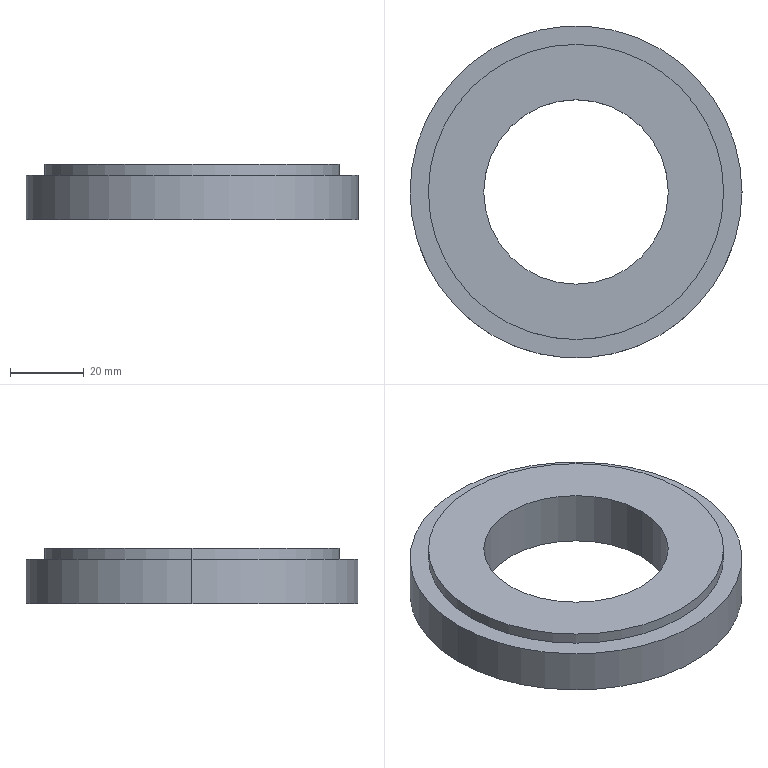Part | SolidWorks | features 3DProfileFeature 1, Extrusion 1, HoleWzd 1, ICE 1 | 1 solid | 33 faces | box 90 x 90 x 15 mm | volume 61433 mm3 | cylinder 18 | cone 12 | plane 3 | commonest cylinder face diameters 3.3 x12 50 x2 80 x2 90 x2
STEP:
#1=CARTESIAN_POINT('',(33.693,18.5,10.1));
#2=VERTEX_POINT('',#1);
#3=CARTESIAN_POINT('',(30.393,18.5,10.1));
#4=VERTEX_POINT('',#3);
#5=CARTESIAN_POINT('',(32.043,18.5,10.1));
#6=DIRECTION('',(0.,0.,-1.));
#7=DIRECTION('',(-1.,0.,0.));
#8=AXIS2_PLACEMENT_3D('',#5,#6,#7);
#9=CIRCLE('',#8,1.65);
#10=EDGE_CURVE('',#2,#4,#9,.T.);
#11=ORIENTED_EDGE('',*,*,#10,.F.);
#12=CARTESIAN_POINT('',(33.693,18.5,0.));
#13=VERTEX_POINT('',#12);
#14=CARTESIAN_POINT('',(33.693,18.5,0.));
#15=DIRECTION('',(0.,0.,-1.));
#16=VECTOR('',#15,1000.);
#17=LINE('',#14,#16);
#18=EDGE_CURVE('',#2,#13,#17,.T.);
#19=ORIENTED_EDGE('',*,*,#18,.T.);
#20=CARTESIAN_POINT('',(30.393,18.5,0.));
#21=VERTEX_POINT('',#20);
#22=CARTESIAN_POINT('',(32.043,18.5,0.));
#23=DIRECTION('',(0.,0.,-1.));
#24=DIRECTION('',(-1.,0.,0.));
#25=AXIS2_PLACEMENT_3D('',#22,#23,#24);
#26=CIRCLE('',#25,1.65);
#27=EDGE_CURVE('',#13,#21,#26,.T.);
#28=ORIENTED_EDGE('',*,*,#27,.T.);
#29=CARTESIAN_POINT('',(30.393,18.5,0.));
#30=DIRECTION('',(0.,0.,-1.));
#31=VECTOR('',#30,1000.);
#32=LINE('',#29,#31);
#33=EDGE_CURVE('',#4,#21,#32,.T.);
#34=ORIENTED_EDGE('',*,*,#33,.F.);
#35=EDGE_LOOP('',(#11,#19,#28,#34));
#36=FACE_OUTER_BOUND('',#35,.T.);
#37=CARTESIAN_POINT('',(32.043,18.5,0.));
#38=DIRECTION('',(0.,0.,-1.));
#39=DIRECTION('',(-1.,0.,0.));
#40=AXIS2_PLACEMENT_3D('',#37,#38,#39);
#41=CYLINDRICAL_SURFACE('',#40,1.65);
#42=ADVANCED_FACE('',(#36),#41,.F.);
#43=CARTESIAN_POINT('',(32.043,18.5,11.091));
#44=VERTEX_POINT('',#43);
#45=CARTESIAN_POINT('',(30.393,18.5,10.1));
#46=DIRECTION('',(-0.8572,0.,-0.515));
#47=VECTOR('',#46,1000.);
#48=LINE('',#45,#47);
#49=EDGE_CURVE('',#44,#4,#48,.T.);
#50=ORIENTED_EDGE('',*,*,#49,.F.);
#51=CARTESIAN_POINT('',(33.693,18.5,10.1));
#52=DIRECTION('',(0.8572,0.,-0.515));
#53=VECTOR('',#52,1000.);
#54=LINE('',#51,#53);
#55=EDGE_CURVE('',#44,#2,#54,.T.);
#56=ORIENTED_EDGE('',*,*,#55,.T.);
#57=ORIENTED_EDGE('',*,*,#10,.T.);
#58=EDGE_LOOP('',(#50,#56,#57));
#59=FACE_OUTER_BOUND('',#58,.T.);
#60=CARTESIAN_POINT('',(32.043,18.5,10.1));
#61=DIRECTION('',(0.,0.,-1.));
#62=DIRECTION('',(-1.,0.,0.));
#63=AXIS2_PLACEMENT_3D('',#60,#61,#62);
#64=CONICAL_SURFACE('',#63,1.65,1.03);
#65=ADVANCED_FACE('',(#59),#64,.F.);
#66=CARTESIAN_POINT('',(1.65,37.,10.1));
#67=VERTEX_POINT('',#66);
#68=CARTESIAN_POINT('',(-1.65,37.,10.1));
#69=VERTEX_POINT('',#68);
#70=CARTESIAN_POINT('',(0.,37.,10.1));
#71=DIRECTION('',(0.,0.,-1.));
#72=DIRECTION('',(-1.,0.,0.));
#73=AXIS2_PLACEMENT_3D('',#70,#71,#72);
#74=CIRCLE('',#73,1.65);
#75=EDGE_CURVE('',#67,#69,#74,.T.);
#76=ORIENTED_EDGE('',*,*,#75,.F.);
#77=CARTESIAN_POINT('',(1.65,37.,0.));
#78=VERTEX_POINT('',#77);
#79=CARTESIAN_POINT('',(1.65,37.,0.));
#80=DIRECTION('',(0.,0.,-1.));
#81=VECTOR('',#80,1000.);
#82=LINE('',#79,#81);
#83=EDGE_CURVE('',#67,#78,#82,.T.);
#84=ORIENTED_EDGE('',*,*,#83,.T.);
#85=CARTESIAN_POINT('',(-1.65,37.,0.));
#86=VERTEX_POINT('',#85);
#87=CARTESIAN_POINT('',(0.,37.,0.));
#88=DIRECTION('',(0.,0.,-1.));
#89=DIRECTION('',(-1.,0.,0.));
#90=AXIS2_PLACEMENT_3D('',#87,#88,#89);
#91=CIRCLE('',#90,1.65);
#92=EDGE_CURVE('',#78,#86,#91,.T.);
#93=ORIENTED_EDGE('',*,*,#92,.T.);
#94=CARTESIAN_POINT('',(-1.65,37.,0.));
#95=DIRECTION('',(0.,0.,-1.));
#96=VECTOR('',#95,1000.);
#97=LINE('',#94,#96);
#98=EDGE_CURVE('',#69,#86,#97,.T.);
#99=ORIENTED_EDGE('',*,*,#98,.F.);
#100=EDGE_LOOP('',(#76,#84,#93,#99));
#101=FACE_OUTER_BOUND('',#100,.T.);
#102=CARTESIAN_POINT('',(0.,37.,0.));
#103=DIRECTION('',(0.,0.,-1.));
#104=DIRECTION('',(-1.,0.,0.));
#105=AXIS2_PLACEMENT_3D('',#102,#103,#104);
#106=CYLINDRICAL_SURFACE('',#105,1.65);
#107=ADVANCED_FACE('',(#101),#106,.F.);
#108=CARTESIAN_POINT('',(0.,37.,11.091));
#109=VERTEX_POINT('',#108);
#110=CARTESIAN_POINT('',(-1.65,37.,10.1));
#111=DIRECTION('',(-0.8572,0.,-0.515));
#112=VECTOR('',#111,1000.);
#113=LINE('',#110,#112);
#114=EDGE_CURVE('',#109,#69,#113,.T.);
#115=ORIENTED_EDGE('',*,*,#114,.F.);
#116=CARTESIAN_POINT('',(1.65,37.,10.1));
#117=DIRECTION('',(0.8572,0.,-0.515));
#118=VECTOR('',#117,1000.);
#119=LINE('',#116,#118);
#120=EDGE_CURVE('',#109,#67,#119,.T.);
#121=ORIENTED_EDGE('',*,*,#120,.T.);
#122=ORIENTED_EDGE('',*,*,#75,.T.);
#123=EDGE_LOOP('',(#115,#121,#122));
#124=FACE_OUTER_BOUND('',#123,.T.);
#125=CARTESIAN_POINT('',(0.,37.,10.1));
#126=DIRECTION('',(0.,0.,-1.));
#127=DIRECTION('',(-1.,0.,0.));
#128=AXIS2_PLACEMENT_3D('',#125,#126,#127);
#129=CONICAL_SURFACE('',#128,1.65,1.03);
#130=ADVANCED_FACE('',(#124),#129,.F.);
#131=CARTESIAN_POINT('',(-30.393,18.5,10.1));
#132=VERTEX_POINT('',#131);
#133=CARTESIAN_POINT('',(-33.693,18.5,10.1));
#134=VERTEX_POINT('',#133);
#135=CARTESIAN_POINT('',(-32.043,18.5,10.1));
#136=DIRECTION('',(0.,0.,-1.));
#137=DIRECTION('',(-1.,0.,0.));
#138=AXIS2_PLACEMENT_3D('',#135,#136,#137);
#139=CIRCLE('',#138,1.65);
#140=EDGE_CURVE('',#132,#134,#139,.T.);
#141=ORIENTED_EDGE('',*,*,#140,.F.);
#142=CARTESIAN_POINT('',(-30.393,18.5,0.));
#143=VERTEX_POINT('',#142);
#144=CARTESIAN_POINT('',(-30.393,18.5,0.));
#145=DIRECTION('',(0.,0.,-1.));
#146=VECTOR('',#145,1000.);
#147=LINE('',#144,#146);
#148=EDGE_CURVE('',#132,#143,#147,.T.);
#149=ORIENTED_EDGE('',*,*,#148,.T.);
#150=CARTESIAN_POINT('',(-33.693,18.5,0.));
#151=VERTEX_POINT('',#150);
#152=CARTESIAN_POINT('',(-32.043,18.5,0.));
#153=DIRECTION('',(0.,0.,-1.));
#154=DIRECTION('',(-1.,0.,0.));
#155=AXIS2_PLACEMENT_3D('',#152,#153,#154);
#156=CIRCLE('',#155,1.65);
#157=EDGE_CURVE('',#143,#151,#156,.T.);
#158=ORIENTED_EDGE('',*,*,#157,.T.);
#159=CARTESIAN_POINT('',(-33.693,18.5,0.));
#160=DIRECTION('',(0.,0.,-1.));
#161=VECTOR('',#160,1000.);
#162=LINE('',#159,#161);
#163=EDGE_CURVE('',#134,#151,#162,.T.);
#164=ORIENTED_EDGE('',*,*,#163,.F.);
#165=EDGE_LOOP('',(#141,#149,#158,#164));
#166=FACE_OUTER_BOUND('',#165,.T.);
#167=CARTESIAN_POINT('',(-32.043,18.5,0.));
#168=DIRECTION('',(0.,0.,-1.));
#169=DIRECTION('',(-1.,0.,0.));
#170=AXIS2_PLACEMENT_3D('',#167,#168,#169);
#171=CYLINDRICAL_SURFACE('',#170,1.65);
#172=ADVANCED_FACE('',(#166),#171,.F.);
#173=CARTESIAN_POINT('',(-32.043,18.5,11.091));
#174=VERTEX_POINT('',#173);
#175=CARTESIAN_POINT('',(-33.693,18.5,10.1));
#176=DIRECTION('',(-0.8572,0.,-0.515));
#177=VECTOR('',#176,1000.);
#178=LINE('',#175,#177);
#179=EDGE_CURVE('',#174,#134,#178,.T.);
#180=ORIENTED_EDGE('',*,*,#179,.F.);
#181=CARTESIAN_POINT('',(-30.393,18.5,10.1));
#182=DIRECTION('',(0.8572,0.,-0.515));
#183=VECTOR('',#182,1000.);
#184=LINE('',#181,#183);
#185=EDGE_CURVE('',#174,#132,#184,.T.);
#186=ORIENTED_EDGE('',*,*,#185,.T.);
#187=ORIENTED_EDGE('',*,*,#140,.T.);
#188=EDGE_LOOP('',(#180,#186,#187));
#189=FACE_OUTER_BOUND('',#188,.T.);
#190=CARTESIAN_POINT('',(-32.043,18.5,10.1));
#191=DIRECTION('',(0.,0.,-1.));
#192=DIRECTION('',(-1.,0.,0.));
#193=AXIS2_PLACEMENT_3D('',#190,#191,#192);
#194=CONICAL_SURFACE('',#193,1.65,1.03);
#195=ADVANCED_FACE('',(#189),#194,.F.);
#196=CARTESIAN_POINT('',(-30.393,-18.5,10.1));
#197=VERTEX_POINT('',#196);
#198=CARTESIAN_POINT('',(-33.693,-18.5,10.1));
#199=VERTEX_POINT('',#198);
#200=CARTESIAN_POINT('',(-32.043,-18.5,10.1));
#201=DIRECTION('',(0.,0.,-1.));
#202=DIRECTION('',(-1.,0.,0.));
#203=AXIS2_PLACEMENT_3D('',#200,#201,#202);
#204=CIRCLE('',#203,1.65);
#205=EDGE_CURVE('',#197,#199,#204,.T.);
#206=ORIENTED_EDGE('',*,*,#205,.F.);
#207=CARTESIAN_POINT('',(-30.393,-18.5,0.));
#208=VERTEX_POINT('',#207);
#209=CARTESIAN_POINT('',(-30.393,-18.5,0.));
#210=DIRECTION('',(0.,0.,-1.));
#211=VECTOR('',#210,1000.);
#212=LINE('',#209,#211);
#213=EDGE_CURVE('',#197,#208,#212,.T.);
#214=ORIENTED_EDGE('',*,*,#213,.T.);
#215=CARTESIAN_POINT('',(-33.693,-18.5,0.));
#216=VERTEX_POINT('',#215);
#217=CARTESIAN_POINT('',(-32.043,-18.5,0.));
#218=DIRECTION('',(0.,0.,-1.));
#219=DIRECTION('',(-1.,0.,0.));
#220=AXIS2_PLACEMENT_3D('',#217,#218,#219);
#221=CIRCLE('',#220,1.65);
#222=EDGE_CURVE('',#208,#216,#221,.T.);
#223=ORIENTED_EDGE('',*,*,#222,.T.);
#224=CARTESIAN_POINT('',(-33.693,-18.5,0.));
#225=DIRECTION('',(0.,0.,-1.));
#226=VECTOR('',#225,1000.);
#227=LINE('',#224,#226);
#228=EDGE_CURVE('',#199,#216,#227,.T.);
#229=ORIENTED_EDGE('',*,*,#228,.F.);
#230=EDGE_LOOP('',(#206,#214,#223,#229));
#231=FACE_OUTER_BOUND('',#230,.T.);
#232=CARTESIAN_POINT('',(-32.043,-18.5,0.));
#233=DIRECTION('',(0.,0.,-1.));
#234=DIRECTION('',(-1.,0.,0.));
#235=AXIS2_PLACEMENT_3D('',#232,#233,#234);
#236=CYLINDRICAL_SURFACE('',#235,1.65);
#237=ADVANCED_FACE('',(#231),#236,.F.);
#238=CARTESIAN_POINT('',(-32.043,-18.5,11.091));
#239=VERTEX_POINT('',#238);
#240=CARTESIAN_POINT('',(-33.693,-18.5,10.1));
#241=DIRECTION('',(-0.8572,0.,-0.515));
#242=VECTOR('',#241,1000.);
#243=LINE('',#240,#242);
#244=EDGE_CURVE('',#239,#199,#243,.T.);
#245=ORIENTED_EDGE('',*,*,#244,.F.);
#246=CARTESIAN_POINT('',(-30.393,-18.5,10.1));
#247=DIRECTION('',(0.8572,0.,-0.515));
#248=VECTOR('',#247,1000.);
#249=LINE('',#246,#248);
#250=EDGE_CURVE('',#239,#197,#249,.T.);
#251=ORIENTED_EDGE('',*,*,#250,.T.);
#252=ORIENTED_EDGE('',*,*,#205,.T.);
#253=EDGE_LOOP('',(#245,#251,#252));
#254=FACE_OUTER_BOUND('',#253,.T.);
#255=CARTESIAN_POINT('',(-32.043,-18.5,10.1));
#256=DIRECTION('',(0.,0.,-1.));
#257=DIRECTION('',(-1.,0.,0.));
#258=AXIS2_PLACEMENT_3D('',#255,#256,#257);
#259=CONICAL_SURFACE('',#258,1.65,1.03);
#260=ADVANCED_FACE('',(#254),#259,.F.);
#261=CARTESIAN_POINT('',(1.65,-37.,10.1));
#262=VERTEX_POINT('',#261);
#263=CARTESIAN_POINT('',(-1.65,-37.,10.1));
#264=VERTEX_POINT('',#263);
#265=CARTESIAN_POINT('',(0.,-37.,10.1));
#266=DIRECTION('',(0.,0.,-1.));
#267=DIRECTION('',(-1.,0.,0.));
#268=AXIS2_PLACEMENT_3D('',#265,#266,#267);
#269=CIRCLE('',#268,1.65);
#270=EDGE_CURVE('',#262,#264,#269,.T.);
#271=ORIENTED_EDGE('',*,*,#270,.F.);
#272=CARTESIAN_POINT('',(1.65,-37.,0.));
#273=VERTEX_POINT('',#272);
#274=CARTESIAN_POINT('',(1.65,-37.,0.));
#275=DIRECTION('',(0.,0.,-1.));
#276=VECTOR('',#275,1000.);
#277=LINE('',#274,#276);
#278=EDGE_CURVE('',#262,#273,#277,.T.);
#279=ORIENTED_EDGE('',*,*,#278,.T.);
#280=CARTESIAN_POINT('',(-1.65,-37.,0.));
#281=VERTEX_POINT('',#280);
#282=CARTESIAN_POINT('',(0.,-37.,0.));
#283=DIRECTION('',(0.,0.,-1.));
#284=DIRECTION('',(-1.,0.,0.));
#285=AXIS2_PLACEMENT_3D('',#282,#283,#284);
#286=CIRCLE('',#285,1.65);
#287=EDGE_CURVE('',#273,#281,#286,.T.);
#288=ORIENTED_EDGE('',*,*,#287,.T.);
#289=CARTESIAN_POINT('',(-1.65,-37.,0.));
#290=DIRECTION('',(0.,0.,-1.));
#291=VECTOR('',#290,1000.);
#292=LINE('',#289,#291);
#293=EDGE_CURVE('',#264,#281,#292,.T.);
#294=ORIENTED_EDGE('',*,*,#293,.F.);
#295=EDGE_LOOP('',(#271,#279,#288,#294));
#296=FACE_OUTER_BOUND('',#295,.T.);
#297=CARTESIAN_POINT('',(0.,-37.,0.));
#298=DIRECTION('',(0.,0.,-1.));
#299=DIRECTION('',(-1.,0.,0.));
#300=AXIS2_PLACEMENT_3D('',#297,#298,#299);
#301=CYLINDRICAL_SURFACE('',#300,1.65);
#302=ADVANCED_FACE('',(#296),#301,.F.);
#303=CARTESIAN_POINT('',(0.,-37.,11.091));
#304=VERTEX_POINT('',#303);
#305=CARTESIAN_POINT('',(-1.65,-37.,10.1));
#306=DIRECTION('',(-0.8572,0.,-0.515));
#307=VECTOR('',#306,1000.);
#308=LINE('',#305,#307);
#309=EDGE_CURVE('',#304,#264,#308,.T.);
#310=ORIENTED_EDGE('',*,*,#309,.F.);
#311=CARTESIAN_POINT('',(1.65,-37.,10.1));
#312=DIRECTION('',(0.8572,0.,-0.515));
#313=VECTOR('',#312,1000.);
#314=LINE('',#311,#313);
#315=EDGE_CURVE('',#304,#262,#314,.T.);
#316=ORIENTED_EDGE('',*,*,#315,.T.);
#317=ORIENTED_EDGE('',*,*,#270,.T.);
#318=EDGE_LOOP('',(#310,#316,#317));
#319=FACE_OUTER_BOUND('',#318,.T.);
#320=CARTESIAN_POINT('',(0.,-37.,10.1));
#321=DIRECTION('',(0.,0.,-1.));
#322=DIRECTION('',(-1.,0.,0.));
#323=AXIS2_PLACEMENT_3D('',#320,#321,#322);
#324=CONICAL_SURFACE('',#323,1.65,1.03);
#325=ADVANCED_FACE('',(#319),#324,.F.);
#326=CARTESIAN_POINT('',(33.693,-18.5,10.1));
#327=VERTEX_POINT('',#326);
#328=CARTESIAN_POINT('',(30.393,-18.5,10.1));
#329=VERTEX_POINT('',#328);
#330=CARTESIAN_POINT('',(32.043,-18.5,10.1));
#331=DIRECTION('',(0.,0.,-1.));
#332=DIRECTION('',(-1.,0.,0.));
#333=AXIS2_PLACEMENT_3D('',#330,#331,#332);
#334=CIRCLE('',#333,1.65);
#335=EDGE_CURVE('',#327,#329,#334,.T.);
#336=ORIENTED_EDGE('',*,*,#335,.F.);
#337=CARTESIAN_POINT('',(33.693,-18.5,0.));
#338=VERTEX_POINT('',#337);
#339=CARTESIAN_POINT('',(33.693,-18.5,0.));
#340=DIRECTION('',(0.,0.,-1.));
#341=VECTOR('',#340,1000.);
#342=LINE('',#339,#341);
#343=EDGE_CURVE('',#327,#338,#342,.T.);
#344=ORIENTED_EDGE('',*,*,#343,.T.);
#345=CARTESIAN_POINT('',(30.393,-18.5,0.));
#346=VERTEX_POINT('',#345);
#347=CARTESIAN_POINT('',(32.043,-18.5,0.));
#348=DIRECTION('',(0.,0.,-1.));
#349=DIRECTION('',(-1.,0.,0.));
#350=AXIS2_PLACEMENT_3D('',#347,#348,#349);
#351=CIRCLE('',#350,1.65);
#352=EDGE_CURVE('',#338,#346,#351,.T.);
#353=ORIENTED_EDGE('',*,*,#352,.T.);
#354=CARTESIAN_POINT('',(30.393,-18.5,0.));
#355=DIRECTION('',(0.,0.,-1.));
#356=VECTOR('',#355,1000.);
#357=LINE('',#354,#356);
#358=EDGE_CURVE('',#329,#346,#357,.T.);
#359=ORIENTED_EDGE('',*,*,#358,.F.);
#360=EDGE_LOOP('',(#336,#344,#353,#359));
#361=FACE_OUTER_BOUND('',#360,.T.);
#362=CARTESIAN_POINT('',(32.043,-18.5,0.));
#363=DIRECTION('',(0.,0.,-1.));
#364=DIRECTION('',(-1.,0.,0.));
#365=AXIS2_PLACEMENT_3D('',#362,#363,#364);
#366=CYLINDRICAL_SURFACE('',#365,1.65);
#367=ADVANCED_FACE('',(#361),#366,.F.);
#368=CARTESIAN_POINT('',(32.043,-18.5,11.091));
#369=VERTEX_POINT('',#368);
#370=CARTESIAN_POINT('',(30.393,-18.5,10.1));
#371=DIRECTION('',(-0.8572,0.,-0.515));
#372=VECTOR('',#371,1000.);
#373=LINE('',#370,#372);
#374=EDGE_CURVE('',#369,#329,#373,.T.);
#375=ORIENTED_EDGE('',*,*,#374,.F.);
#376=CARTESIAN_POINT('',(33.693,-18.5,10.1));
#377=DIRECTION('',(0.8572,0.,-0.515));
#378=VECTOR('',#377,1000.);
#379=LINE('',#376,#378);
#380=EDGE_CURVE('',#369,#327,#379,.T.);
#381=ORIENTED_EDGE('',*,*,#380,.T.);
#382=ORIENTED_EDGE('',*,*,#335,.T.);
#383=EDGE_LOOP('',(#375,#381,#382));
#384=FACE_OUTER_BOUND('',#383,.T.);
#385=CARTESIAN_POINT('',(32.043,-18.5,10.1));
#386=DIRECTION('',(0.,0.,-1.));
#387=DIRECTION('',(-1.,0.,0.));
#388=AXIS2_PLACEMENT_3D('',#385,#386,#387);
#389=CONICAL_SURFACE('',#388,1.65,1.03);
#390=ADVANCED_FACE('',(#384),#389,.F.);
#391=CARTESIAN_POINT('',(40.,0.,15.));
#392=VERTEX_POINT('',#391);
#393=CARTESIAN_POINT('',(-40.,0.,15.));
#394=VERTEX_POINT('',#393);
#395=CARTESIAN_POINT('',(0.,0.,15.));
#396=DIRECTION('',(0.,0.,1.));
#397=DIRECTION('',(1.,0.,0.));
#398=AXIS2_PLACEMENT_3D('',#395,#396,#397);
#399=CIRCLE('',#398,40.);
#400=EDGE_CURVE('',#392,#394,#399,.T.);
#401=ORIENTED_EDGE('',*,*,#400,.F.);
#402=CARTESIAN_POINT('',(40.,0.,12.));
#403=VERTEX_POINT('',#402);
#404=CARTESIAN_POINT('',(40.,0.,15.));
#405=DIRECTION('',(0.,0.,-1.));
#406=VECTOR('',#405,1000.);
#407=LINE('',#404,#406);
#408=EDGE_CURVE('',#392,#403,#407,.T.);
#409=ORIENTED_EDGE('',*,*,#408,.T.);
#410=CARTESIAN_POINT('',(-40.,0.,12.));
#411=VERTEX_POINT('',#410);
#412=CARTESIAN_POINT('',(0.,0.,12.));
#413=DIRECTION('',(0.,0.,1.));
#414=DIRECTION('',(1.,0.,0.));
#415=AXIS2_PLACEMENT_3D('',#412,#413,#414);
#416=CIRCLE('',#415,40.);
#417=EDGE_CURVE('',#403,#411,#416,.T.);
#418=ORIENTED_EDGE('',*,*,#417,.T.);
#419=CARTESIAN_POINT('',(-40.,0.,15.));
#420=DIRECTION('',(0.,0.,-1.));
#421=VECTOR('',#420,1000.);
#422=LINE('',#419,#421);
#423=EDGE_CURVE('',#394,#411,#422,.T.);
#424=ORIENTED_EDGE('',*,*,#423,.F.);
#425=EDGE_LOOP('',(#401,#409,#418,#424));
#426=FACE_OUTER_BOUND('',#425,.T.);
#427=CARTESIAN_POINT('',(0.,0.,15.));
#428=DIRECTION('',(0.,0.,-1.));
#429=DIRECTION('',(-1.,0.,0.));
#430=AXIS2_PLACEMENT_3D('',#427,#428,#429);
#431=CYLINDRICAL_SURFACE('',#430,40.);
#432=ADVANCED_FACE('',(#426),#431,.T.);
#433=CARTESIAN_POINT('',(-25.,0.,15.));
#434=VERTEX_POINT('',#433);
#435=CARTESIAN_POINT('',(25.,0.,15.));
#436=VERTEX_POINT('',#435);
#437=CARTESIAN_POINT('',(0.,0.,15.));
#438=DIRECTION('',(0.,0.,1.));
#439=DIRECTION('',(1.,0.,0.));
#440=AXIS2_PLACEMENT_3D('',#437,#438,#439);
#441=CIRCLE('',#440,25.);
#442=EDGE_CURVE('',#434,#436,#441,.T.);
#443=ORIENTED_EDGE('',*,*,#442,.T.);
#444=CARTESIAN_POINT('',(25.,0.,0.));
#445=VERTEX_POINT('',#444);
#446=CARTESIAN_POINT('',(25.,0.,12.));
#447=DIRECTION('',(0.,0.,-1.));
#448=VECTOR('',#447,1000.);
#449=LINE('',#446,#448);
#450=EDGE_CURVE('',#436,#445,#449,.T.);
#451=ORIENTED_EDGE('',*,*,#450,.T.);
#452=CARTESIAN_POINT('',(-25.,0.,0.));
#453=VERTEX_POINT('',#452);
#454=CARTESIAN_POINT('',(0.,0.,0.));
#455=DIRECTION('',(0.,0.,1.));
#456=DIRECTION('',(1.,0.,0.));
#457=AXIS2_PLACEMENT_3D('',#454,#455,#456);
#458=CIRCLE('',#457,25.);
#459=EDGE_CURVE('',#453,#445,#458,.T.);
#460=ORIENTED_EDGE('',*,*,#459,.F.);
#461=CARTESIAN_POINT('',(-25.,0.,12.));
#462=DIRECTION('',(0.,0.,-1.));
#463=VECTOR('',#462,1000.);
#464=LINE('',#461,#463);
#465=EDGE_CURVE('',#434,#453,#464,.T.);
#466=ORIENTED_EDGE('',*,*,#465,.F.);
#467=EDGE_LOOP('',(#443,#451,#460,#466));
#468=FACE_OUTER_BOUND('',#467,.T.);
#469=CARTESIAN_POINT('',(0.,0.,12.));
#470=DIRECTION('',(0.,0.,-1.));
#471=DIRECTION('',(-1.,0.,0.));
#472=AXIS2_PLACEMENT_3D('',#469,#470,#471);
#473=CYLINDRICAL_SURFACE('',#472,25.);
#474=ADVANCED_FACE('',(#468),#473,.F.);
#475=CARTESIAN_POINT('',(45.,0.,12.));
#476=VERTEX_POINT('',#475);
#477=CARTESIAN_POINT('',(-45.,0.,12.));
#478=VERTEX_POINT('',#477);
#479=CARTESIAN_POINT('',(0.,0.,12.));
#480=DIRECTION('',(0.,0.,1.));
#481=DIRECTION('',(1.,0.,0.));
#482=AXIS2_PLACEMENT_3D('',#479,#480,#481);
#483=CIRCLE('',#482,45.);
#484=EDGE_CURVE('',#476,#478,#483,.T.);
#485=ORIENTED_EDGE('',*,*,#484,.F.);
#486=CARTESIAN_POINT('',(45.,0.,0.));
#487=VERTEX_POINT('',#486);
#488=CARTESIAN_POINT('',(45.,0.,12.));
#489=DIRECTION('',(0.,0.,-1.));
#490=VECTOR('',#489,1000.);
#491=LINE('',#488,#490);
#492=EDGE_CURVE('',#476,#487,#491,.T.);
#493=ORIENTED_EDGE('',*,*,#492,.T.);
#494=CARTESIAN_POINT('',(-45.,0.,0.));
#495=VERTEX_POINT('',#494);
#496=CARTESIAN_POINT('',(0.,0.,0.));
#497=DIRECTION('',(0.,0.,1.));
#498=DIRECTION('',(1.,0.,0.));
#499=AXIS2_PLACEMENT_3D('',#496,#497,#498);
#500=CIRCLE('',#499,45.);
#501=EDGE_CURVE('',#487,#495,#500,.T.);
#502=ORIENTED_EDGE('',*,*,#501,.T.);
#503=CARTESIAN_POINT('',(-45.,0.,12.));
#504=DIRECTION('',(0.,0.,-1.));
#505=VECTOR('',#504,1000.);
#506=LINE('',#503,#505);
#507=EDGE_CURVE('',#478,#495,#506,.T.);
#508=ORIENTED_EDGE('',*,*,#507,.F.);
#509=EDGE_LOOP('',(#485,#493,#502,#508));
#510=FACE_OUTER_BOUND('',#509,.T.);
#511=CARTESIAN_POINT('',(0.,0.,12.));
#512=DIRECTION('',(0.,0.,-1.));
#513=DIRECTION('',(-1.,0.,0.));
#514=AXIS2_PLACEMENT_3D('',#511,#512,#513);
#515=CYLINDRICAL_SURFACE('',#514,45.);
#516=ADVANCED_FACE('',(#510),#515,.T.);
#517=CARTESIAN_POINT('',(0.,0.,12.));
#518=DIRECTION('',(0.,0.,1.));
#519=DIRECTION('',(1.,0.,0.));
#520=AXIS2_PLACEMENT_3D('',#517,#518,#519);
#521=CIRCLE('',#520,45.);
#522=EDGE_CURVE('',#478,#476,#521,.T.);
#523=ORIENTED_EDGE('',*,*,#522,.T.);
#524=ORIENTED_EDGE('',*,*,#484,.T.);
#525=EDGE_LOOP('',(#523,#524));
#526=FACE_OUTER_BOUND('',#525,.T.);
#527=CARTESIAN_POINT('',(0.,0.,12.));
#528=DIRECTION('',(0.,0.,1.));
#529=DIRECTION('',(1.,0.,0.));
#530=AXIS2_PLACEMENT_3D('',#527,#528,#529);
#531=CIRCLE('',#530,40.);
#532=EDGE_CURVE('',#411,#403,#531,.T.);
#533=ORIENTED_EDGE('',*,*,#532,.F.);
#534=ORIENTED_EDGE('',*,*,#417,.F.);
#535=EDGE_LOOP('',(#533,#534));
#536=FACE_BOUND('',#535,.T.);
#537=CARTESIAN_POINT('',(0.,0.,12.));
#538=DIRECTION('',(0.,0.,1.));
#539=DIRECTION('',(1.,0.,0.));
#540=AXIS2_PLACEMENT_3D('',#537,#538,#539);
#541=PLANE('',#540);
#542=ADVANCED_FACE('',(#526,#536),#541,.T.);
#543=CARTESIAN_POINT('',(32.043,18.5,0.));
#544=DIRECTION('',(0.,0.,-1.));
#545=DIRECTION('',(-1.,0.,0.));
#546=AXIS2_PLACEMENT_3D('',#543,#544,#545);
#547=CIRCLE('',#546,1.65);
#548=EDGE_CURVE('',#21,#13,#547,.T.);
#549=ORIENTED_EDGE('',*,*,#548,.F.);
#550=ORIENTED_EDGE('',*,*,#27,.F.);
#551=EDGE_LOOP('',(#549,#550));
#552=FACE_BOUND('',#551,.T.);
#553=CARTESIAN_POINT('',(0.,37.,0.));
#554=DIRECTION('',(0.,0.,-1.));
#555=DIRECTION('',(-1.,0.,0.));
#556=AXIS2_PLACEMENT_3D('',#553,#554,#555);
#557=CIRCLE('',#556,1.65);
#558=EDGE_CURVE('',#86,#78,#557,.T.);
#559=ORIENTED_EDGE('',*,*,#558,.F.);
#560=ORIENTED_EDGE('',*,*,#92,.F.);
#561=EDGE_LOOP('',(#559,#560));
#562=FACE_BOUND('',#561,.T.);
#563=CARTESIAN_POINT('',(-32.043,18.5,0.));
#564=DIRECTION('',(0.,0.,-1.));
#565=DIRECTION('',(-1.,0.,0.));
#566=AXIS2_PLACEMENT_3D('',#563,#564,#565);
#567=CIRCLE('',#566,1.65);
#568=EDGE_CURVE('',#151,#143,#567,.T.);
#569=ORIENTED_EDGE('',*,*,#568,.F.);
#570=ORIENTED_EDGE('',*,*,#157,.F.);
#571=EDGE_LOOP('',(#569,#570));
#572=FACE_BOUND('',#571,.T.);
#573=CARTESIAN_POINT('',(-32.043,-18.5,0.));
#574=DIRECTION('',(0.,0.,-1.));
#575=DIRECTION('',(-1.,0.,0.));
#576=AXIS2_PLACEMENT_3D('',#573,#574,#575);
#577=CIRCLE('',#576,1.65);
#578=EDGE_CURVE('',#216,#208,#577,.T.);
#579=ORIENTED_EDGE('',*,*,#578,.F.);
#580=ORIENTED_EDGE('',*,*,#222,.F.);
#581=EDGE_LOOP('',(#579,#580));
#582=FACE_BOUND('',#581,.T.);
#583=CARTESIAN_POINT('',(0.,-37.,0.));
#584=DIRECTION('',(0.,0.,-1.));
#585=DIRECTION('',(-1.,0.,0.));
#586=AXIS2_PLACEMENT_3D('',#583,#584,#585);
#587=CIRCLE('',#586,1.65);
#588=EDGE_CURVE('',#281,#273,#587,.T.);
#589=ORIENTED_EDGE('',*,*,#588,.F.);
#590=ORIENTED_EDGE('',*,*,#287,.F.);
#591=EDGE_LOOP('',(#589,#590));
#592=FACE_BOUND('',#591,.T.);
#593=CARTESIAN_POINT('',(32.043,-18.5,0.));
#594=DIRECTION('',(0.,0.,-1.));
#595=DIRECTION('',(-1.,0.,0.));
#596=AXIS2_PLACEMENT_3D('',#593,#594,#595);
#597=CIRCLE('',#596,1.65);
#598=EDGE_CURVE('',#346,#338,#597,.T.);
#599=ORIENTED_EDGE('',*,*,#598,.F.);
#600=ORIENTED_EDGE('',*,*,#352,.F.);
#601=EDGE_LOOP('',(#599,#600));
#602=FACE_BOUND('',#601,.T.);
#603=CARTESIAN_POINT('',(0.,0.,0.));
#604=DIRECTION('',(0.,0.,1.));
#605=DIRECTION('',(1.,0.,0.));
#606=AXIS2_PLACEMENT_3D('',#603,#604,#605);
#607=CIRCLE('',#606,45.);
#608=EDGE_CURVE('',#495,#487,#607,.T.);
#609=ORIENTED_EDGE('',*,*,#608,.F.);
#610=ORIENTED_EDGE('',*,*,#501,.F.);
#611=EDGE_LOOP('',(#609,#610));
#612=FACE_OUTER_BOUND('',#611,.T.);
#613=ORIENTED_EDGE('',*,*,#459,.T.);
#614=CARTESIAN_POINT('',(0.,0.,0.));
#615=DIRECTION('',(0.,0.,1.));
#616=DIRECTION('',(1.,0.,0.));
#617=AXIS2_PLACEMENT_3D('',#614,#615,#616);
#618=CIRCLE('',#617,25.);
#619=EDGE_CURVE('',#445,#453,#618,.T.);
#620=ORIENTED_EDGE('',*,*,#619,.T.);
#621=EDGE_LOOP('',(#613,#620));
#622=FACE_BOUND('',#621,.T.);
#623=CARTESIAN_POINT('',(0.,0.,0.));
#624=DIRECTION('',(0.,0.,1.));
#625=DIRECTION('',(1.,0.,0.));
#626=AXIS2_PLACEMENT_3D('',#623,#624,#625);
#627=PLANE('',#626);
#628=ADVANCED_FACE('',(#552,#562,#572,#582,#592,#602,#612,#622),#627,.F.);
#629=ORIENTED_EDGE('',*,*,#492,.F.);
#630=ORIENTED_EDGE('',*,*,#522,.F.);
#631=ORIENTED_EDGE('',*,*,#507,.T.);
#632=ORIENTED_EDGE('',*,*,#608,.T.);
#633=EDGE_LOOP('',(#629,#630,#631,#632));
#634=FACE_OUTER_BOUND('',#633,.T.);
#635=CARTESIAN_POINT('',(0.,0.,12.));
#636=DIRECTION('',(0.,0.,-1.));
#637=DIRECTION('',(-1.,0.,0.));
#638=AXIS2_PLACEMENT_3D('',#635,#636,#637);
#639=CYLINDRICAL_SURFACE('',#638,45.);
#640=ADVANCED_FACE('',(#634),#639,.T.);
#641=ORIENTED_EDGE('',*,*,#450,.F.);
#642=CARTESIAN_POINT('',(0.,0.,15.));
#643=DIRECTION('',(0.,0.,1.));
#644=DIRECTION('',(1.,0.,0.));
#645=AXIS2_PLACEMENT_3D('',#642,#643,#644);
#646=CIRCLE('',#645,25.);
#647=EDGE_CURVE('',#436,#434,#646,.T.);
#648=ORIENTED_EDGE('',*,*,#647,.T.);
#649=ORIENTED_EDGE('',*,*,#465,.T.);
#650=ORIENTED_EDGE('',*,*,#619,.F.);
#651=EDGE_LOOP('',(#641,#648,#649,#650));
#652=FACE_OUTER_BOUND('',#651,.T.);
#653=CARTESIAN_POINT('',(0.,0.,12.));
#654=DIRECTION('',(0.,0.,-1.));
#655=DIRECTION('',(-1.,0.,0.));
#656=AXIS2_PLACEMENT_3D('',#653,#654,#655);
#657=CYLINDRICAL_SURFACE('',#656,25.);
#658=ADVANCED_FACE('',(#652),#657,.F.);
#659=CARTESIAN_POINT('',(0.,0.,15.));
#660=DIRECTION('',(0.,0.,1.));
#661=DIRECTION('',(1.,0.,0.));
#662=AXIS2_PLACEMENT_3D('',#659,#660,#661);
#663=CIRCLE('',#662,40.);
#664=EDGE_CURVE('',#394,#392,#663,.T.);
#665=ORIENTED_EDGE('',*,*,#664,.T.);
#666=ORIENTED_EDGE('',*,*,#400,.T.);
#667=EDGE_LOOP('',(#665,#666));
#668=FACE_OUTER_BOUND('',#667,.T.);
#669=ORIENTED_EDGE('',*,*,#442,.F.);
#670=ORIENTED_EDGE('',*,*,#647,.F.);
#671=EDGE_LOOP('',(#669,#670));
#672=FACE_BOUND('',#671,.T.);
#673=CARTESIAN_POINT('',(0.,0.,15.));
#674=DIRECTION('',(0.,0.,1.));
#675=DIRECTION('',(1.,0.,0.));
#676=AXIS2_PLACEMENT_3D('',#673,#674,#675);
#677=PLANE('',#676);
#678=ADVANCED_FACE('',(#668,#672),#677,.T.);
#679=ORIENTED_EDGE('',*,*,#408,.F.);
#680=ORIENTED_EDGE('',*,*,#664,.F.);
#681=ORIENTED_EDGE('',*,*,#423,.T.);
#682=ORIENTED_EDGE('',*,*,#532,.T.);
#683=EDGE_LOOP('',(#679,#680,#681,#682));
#684=FACE_OUTER_BOUND('',#683,.T.);
#685=CARTESIAN_POINT('',(0.,0.,15.));
#686=DIRECTION('',(0.,0.,-1.));
#687=DIRECTION('',(-1.,0.,0.));
#688=AXIS2_PLACEMENT_3D('',#685,#686,#687);
#689=CYLINDRICAL_SURFACE('',#688,40.);
#690=ADVANCED_FACE('',(#684),#689,.T.);
#691=ORIENTED_EDGE('',*,*,#380,.F.);
#692=ORIENTED_EDGE('',*,*,#374,.T.);
#693=CARTESIAN_POINT('',(32.043,-18.5,10.1));
#694=DIRECTION('',(0.,0.,-1.));
#695=DIRECTION('',(-1.,0.,0.));
#696=AXIS2_PLACEMENT_3D('',#693,#694,#695);
#697=CIRCLE('',#696,1.65);
#698=EDGE_CURVE('',#329,#327,#697,.T.);
#699=ORIENTED_EDGE('',*,*,#698,.T.);
#700=EDGE_LOOP('',(#691,#692,#699));
#701=FACE_OUTER_BOUND('',#700,.T.);
#702=CARTESIAN_POINT('',(32.043,-18.5,10.1));
#703=DIRECTION('',(0.,0.,-1.));
#704=DIRECTION('',(-1.,0.,0.));
#705=AXIS2_PLACEMENT_3D('',#702,#703,#704);
#706=CONICAL_SURFACE('',#705,1.65,1.03);
#707=ADVANCED_FACE('',(#701),#706,.F.);
#708=ORIENTED_EDGE('',*,*,#343,.F.);
#709=ORIENTED_EDGE('',*,*,#698,.F.);
#710=ORIENTED_EDGE('',*,*,#358,.T.);
#711=ORIENTED_EDGE('',*,*,#598,.T.);
#712=EDGE_LOOP('',(#708,#709,#710,#711));
#713=FACE_OUTER_BOUND('',#712,.T.);
#714=CARTESIAN_POINT('',(32.043,-18.5,0.));
#715=DIRECTION('',(0.,0.,-1.));
#716=DIRECTION('',(-1.,0.,0.));
#717=AXIS2_PLACEMENT_3D('',#714,#715,#716);
#718=CYLINDRICAL_SURFACE('',#717,1.65);
#719=ADVANCED_FACE('',(#713),#718,.F.);
#720=ORIENTED_EDGE('',*,*,#315,.F.);
#721=ORIENTED_EDGE('',*,*,#309,.T.);
#722=CARTESIAN_POINT('',(0.,-37.,10.1));
#723=DIRECTION('',(0.,0.,-1.));
#724=DIRECTION('',(-1.,0.,0.));
#725=AXIS2_PLACEMENT_3D('',#722,#723,#724);
#726=CIRCLE('',#725,1.65);
#727=EDGE_CURVE('',#264,#262,#726,.T.);
#728=ORIENTED_EDGE('',*,*,#727,.T.);
#729=EDGE_LOOP('',(#720,#721,#728));
#730=FACE_OUTER_BOUND('',#729,.T.);
#731=CARTESIAN_POINT('',(0.,-37.,10.1));
#732=DIRECTION('',(0.,0.,-1.));
#733=DIRECTION('',(-1.,0.,0.));
#734=AXIS2_PLACEMENT_3D('',#731,#732,#733);
#735=CONICAL_SURFACE('',#734,1.65,1.03);
#736=ADVANCED_FACE('',(#730),#735,.F.);
#737=ORIENTED_EDGE('',*,*,#278,.F.);
#738=ORIENTED_EDGE('',*,*,#727,.F.);
#739=ORIENTED_EDGE('',*,*,#293,.T.);
#740=ORIENTED_EDGE('',*,*,#588,.T.);
#741=EDGE_LOOP('',(#737,#738,#739,#740));
#742=FACE_OUTER_BOUND('',#741,.T.);
#743=CARTESIAN_POINT('',(0.,-37.,0.));
#744=DIRECTION('',(0.,0.,-1.));
#745=DIRECTION('',(-1.,0.,0.));
#746=AXIS2_PLACEMENT_3D('',#743,#744,#745);
#747=CYLINDRICAL_SURFACE('',#746,1.65);
#748=ADVANCED_FACE('',(#742),#747,.F.);
#749=ORIENTED_EDGE('',*,*,#250,.F.);
#750=ORIENTED_EDGE('',*,*,#244,.T.);
#751=CARTESIAN_POINT('',(-32.043,-18.5,10.1));
#752=DIRECTION('',(0.,0.,-1.));
#753=DIRECTION('',(-1.,0.,0.));
#754=AXIS2_PLACEMENT_3D('',#751,#752,#753);
#755=CIRCLE('',#754,1.65);
#756=EDGE_CURVE('',#199,#197,#755,.T.);
#757=ORIENTED_EDGE('',*,*,#756,.T.);
#758=EDGE_LOOP('',(#749,#750,#757));
#759=FACE_OUTER_BOUND('',#758,.T.);
#760=CARTESIAN_POINT('',(-32.043,-18.5,10.1));
#761=DIRECTION('',(0.,0.,-1.));
#762=DIRECTION('',(-1.,0.,0.));
#763=AXIS2_PLACEMENT_3D('',#760,#761,#762);
#764=CONICAL_SURFACE('',#763,1.65,1.03);
#765=ADVANCED_FACE('',(#759),#764,.F.);
#766=ORIENTED_EDGE('',*,*,#213,.F.);
#767=ORIENTED_EDGE('',*,*,#756,.F.);
#768=ORIENTED_EDGE('',*,*,#228,.T.);
#769=ORIENTED_EDGE('',*,*,#578,.T.);
#770=EDGE_LOOP('',(#766,#767,#768,#769));
#771=FACE_OUTER_BOUND('',#770,.T.);
#772=CARTESIAN_POINT('',(-32.043,-18.5,0.));
#773=DIRECTION('',(0.,0.,-1.));
#774=DIRECTION('',(-1.,0.,0.));
#775=AXIS2_PLACEMENT_3D('',#772,#773,#774);
#776=CYLINDRICAL_SURFACE('',#775,1.65);
#777=ADVANCED_FACE('',(#771),#776,.F.);
#778=ORIENTED_EDGE('',*,*,#185,.F.);
#779=ORIENTED_EDGE('',*,*,#179,.T.);
#780=CARTESIAN_POINT('',(-32.043,18.5,10.1));
#781=DIRECTION('',(0.,0.,-1.));
#782=DIRECTION('',(-1.,0.,0.));
#783=AXIS2_PLACEMENT_3D('',#780,#781,#782);
#784=CIRCLE('',#783,1.65);
#785=EDGE_CURVE('',#134,#132,#784,.T.);
#786=ORIENTED_EDGE('',*,*,#785,.T.);
#787=EDGE_LOOP('',(#778,#779,#786));
#788=FACE_OUTER_BOUND('',#787,.T.);
#789=CARTESIAN_POINT('',(-32.043,18.5,10.1));
#790=DIRECTION('',(0.,0.,-1.));
#791=DIRECTION('',(-1.,0.,0.));
#792=AXIS2_PLACEMENT_3D('',#789,#790,#791);
#793=CONICAL_SURFACE('',#792,1.65,1.03);
#794=ADVANCED_FACE('',(#788),#793,.F.);
#795=ORIENTED_EDGE('',*,*,#148,.F.);
#796=ORIENTED_EDGE('',*,*,#785,.F.);
#797=ORIENTED_EDGE('',*,*,#163,.T.);
#798=ORIENTED_EDGE('',*,*,#568,.T.);
#799=EDGE_LOOP('',(#795,#796,#797,#798));
#800=FACE_OUTER_BOUND('',#799,.T.);
#801=CARTESIAN_POINT('',(-32.043,18.5,0.));
#802=DIRECTION('',(0.,0.,-1.));
#803=DIRECTION('',(-1.,0.,0.));
#804=AXIS2_PLACEMENT_3D('',#801,#802,#803);
#805=CYLINDRICAL_SURFACE('',#804,1.65);
#806=ADVANCED_FACE('',(#800),#805,.F.);
#807=ORIENTED_EDGE('',*,*,#120,.F.);
#808=ORIENTED_EDGE('',*,*,#114,.T.);
#809=CARTESIAN_POINT('',(0.,37.,10.1));
#810=DIRECTION('',(0.,0.,-1.));
#811=DIRECTION('',(-1.,0.,0.));
#812=AXIS2_PLACEMENT_3D('',#809,#810,#811);
#813=CIRCLE('',#812,1.65);
#814=EDGE_CURVE('',#69,#67,#813,.T.);
#815=ORIENTED_EDGE('',*,*,#814,.T.);
#816=EDGE_LOOP('',(#807,#808,#815));
#817=FACE_OUTER_BOUND('',#816,.T.);
#818=CARTESIAN_POINT('',(0.,37.,10.1));
#819=DIRECTION('',(0.,0.,-1.));
#820=DIRECTION('',(-1.,0.,0.));
#821=AXIS2_PLACEMENT_3D('',#818,#819,#820);
#822=CONICAL_SURFACE('',#821,1.65,1.03);
#823=ADVANCED_FACE('',(#817),#822,.F.);
#824=ORIENTED_EDGE('',*,*,#83,.F.);
#825=ORIENTED_EDGE('',*,*,#814,.F.);
#826=ORIENTED_EDGE('',*,*,#98,.T.);
#827=ORIENTED_EDGE('',*,*,#558,.T.);
#828=EDGE_LOOP('',(#824,#825,#826,#827));
#829=FACE_OUTER_BOUND('',#828,.T.);
#830=CARTESIAN_POINT('',(0.,37.,0.));
#831=DIRECTION('',(0.,0.,-1.));
#832=DIRECTION('',(-1.,0.,0.));
#833=AXIS2_PLACEMENT_3D('',#830,#831,#832);
#834=CYLINDRICAL_SURFACE('',#833,1.65);
#835=ADVANCED_FACE('',(#829),#834,.F.);
#836=ORIENTED_EDGE('',*,*,#55,.F.);
#837=ORIENTED_EDGE('',*,*,#49,.T.);
#838=CARTESIAN_POINT('',(32.043,18.5,10.1));
#839=DIRECTION('',(0.,0.,-1.));
#840=DIRECTION('',(-1.,0.,0.));
#841=AXIS2_PLACEMENT_3D('',#838,#839,#840);
#842=CIRCLE('',#841,1.65);
#843=EDGE_CURVE('',#4,#2,#842,.T.);
#844=ORIENTED_EDGE('',*,*,#843,.T.);
#845=EDGE_LOOP('',(#836,#837,#844));
#846=FACE_OUTER_BOUND('',#845,.T.);
#847=CARTESIAN_POINT('',(32.043,18.5,10.1));
#848=DIRECTION('',(0.,0.,-1.));
#849=DIRECTION('',(-1.,0.,0.));
#850=AXIS2_PLACEMENT_3D('',#847,#848,#849);
#851=CONICAL_SURFACE('',#850,1.65,1.03);
#852=ADVANCED_FACE('',(#846),#851,.F.);
#853=ORIENTED_EDGE('',*,*,#18,.F.);
#854=ORIENTED_EDGE('',*,*,#843,.F.);
#855=ORIENTED_EDGE('',*,*,#33,.T.);
#856=ORIENTED_EDGE('',*,*,#548,.T.);
#857=EDGE_LOOP('',(#853,#854,#855,#856));
#858=FACE_OUTER_BOUND('',#857,.T.);
#859=CARTESIAN_POINT('',(32.043,18.5,0.));
#860=DIRECTION('',(0.,0.,-1.));
#861=DIRECTION('',(-1.,0.,0.));
#862=AXIS2_PLACEMENT_3D('',#859,#860,#861);
#863=CYLINDRICAL_SURFACE('',#862,1.65);
#864=ADVANCED_FACE('',(#858),#863,.F.);
#865=CLOSED_SHELL('',(#42,#65,#107,#130,#172,#195,#237,#260,#302,#325,#367,#390,#432,#474,#516,#542,#628,#640,#658,#678,#690,#707,#719,#736,#748,#765,#777,#794,#806,#823,#835,#852,#864));
#866=MANIFOLD_SOLID_BREP('',#865);
#867=CARTESIAN_POINT('',(0.,0.,0.));
#868=DIRECTION('',(0.,0.,1.));
#869=DIRECTION('',(1.,0.,0.));
#870=AXIS2_PLACEMENT_3D('',#867,#868,#869);
#871=(LENGTH_UNIT()NAMED_UNIT(*)SI_UNIT(.MILLI.,.METRE.));
#872=UNCERTAINTY_MEASURE_WITH_UNIT(LENGTH_MEASURE(0.00001),#871,'','');
#873=(NAMED_UNIT(*)PLANE_ANGLE_UNIT()SI_UNIT($,.RADIAN.));
#874=(NAMED_UNIT(*)SI_UNIT($,.STERADIAN.)SOLID_ANGLE_UNIT());
#875=(GEOMETRIC_REPRESENTATION_CONTEXT(3)GLOBAL_UNCERTAINTY_ASSIGNED_CONTEXT((#872))GLOBAL_UNIT_ASSIGNED_CONTEXT((#871,#873,#874))REPRESENTATION_CONTEXT('',''));
#876=ADVANCED_BREP_SHAPE_REPRESENTATION('',(#866,#870),#875);